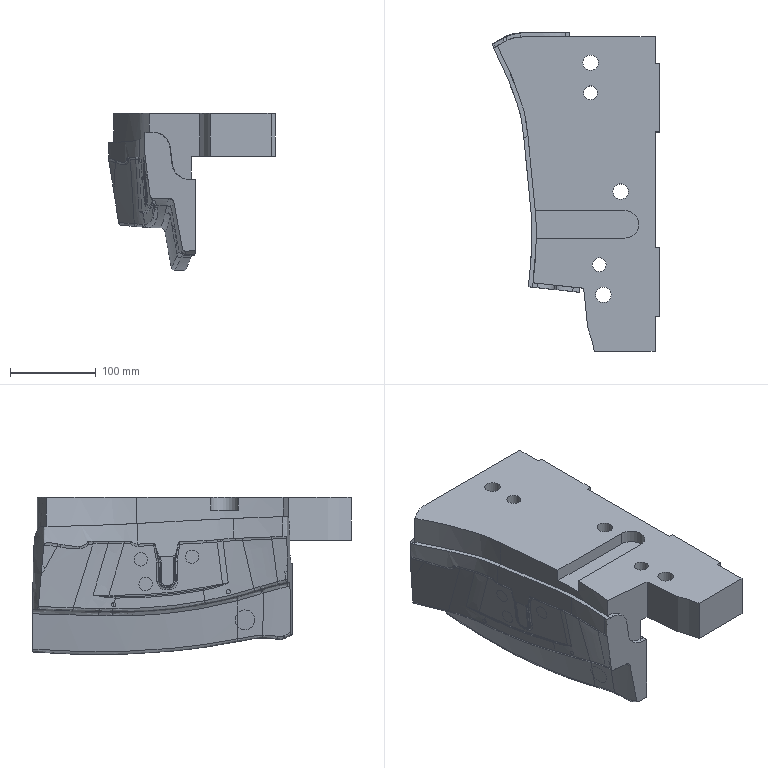Part | NX | features solid 2 | 1 solid | 188 faces | box 193.951 x 370.607 x 182.77 mm | volume 3855927 mm3 | spline 153 | plane 24 | cylinder 11 | commonest cylinder face diameters 18 x3 26 x3 16 x2 40 x2 32 x1